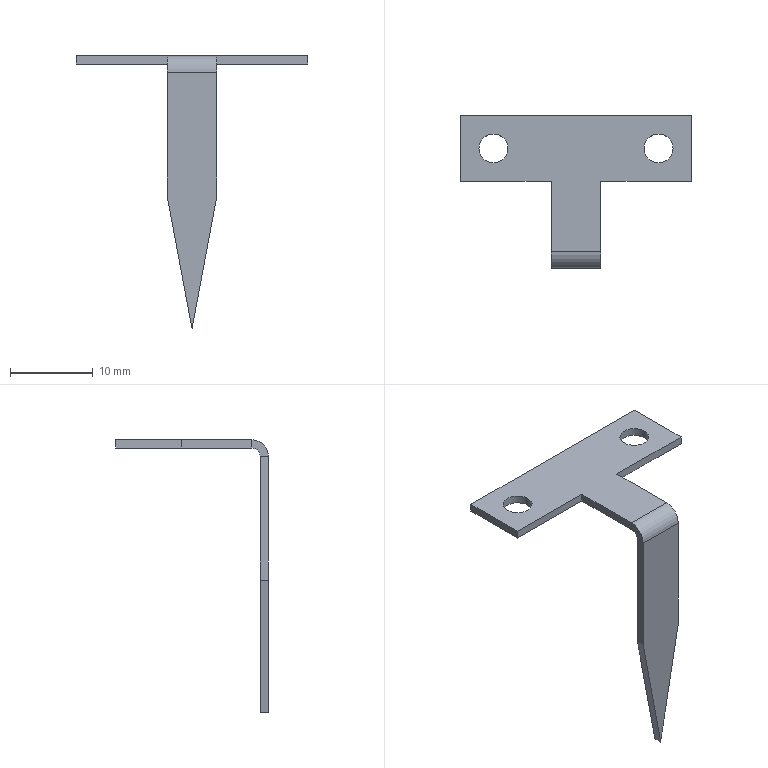Part | SolidWorks | features EdgeFlange 1, FlatPattern 1, SMBaseFlange 1, SheetMetal 1 | 1 solid | 23 faces | box 28 x 18.5 x 33 mm | volume 407.895 mm3 | plane 17 | cylinder 6 | commonest cylinder face diameters 3.5 x4 2 x1 4 x1
STEP:
#1=CARTESIAN_POINT('',(22.25,-4.,-1.));
#2=VERTEX_POINT('',#1);
#3=CARTESIAN_POINT('',(25.75,-4.,-1.));
#4=VERTEX_POINT('',#3);
#5=CARTESIAN_POINT('',(24.,-4.,-1.));
#6=DIRECTION('',(0.,0.,1.));
#7=DIRECTION('',(1.,0.,0.));
#8=AXIS2_PLACEMENT_3D('',#5,#6,#7);
#9=CIRCLE('',#8,1.75);
#10=EDGE_CURVE('',#2,#4,#9,.T.);
#11=ORIENTED_EDGE('',*,*,#10,.F.);
#12=CARTESIAN_POINT('',(22.25,-4.,0.));
#13=VERTEX_POINT('',#12);
#14=CARTESIAN_POINT('',(22.25,-4.,-1.));
#15=DIRECTION('',(0.,0.,1.));
#16=VECTOR('',#15,1000.);
#17=LINE('',#14,#16);
#18=EDGE_CURVE('',#2,#13,#17,.T.);
#19=ORIENTED_EDGE('',*,*,#18,.T.);
#20=CARTESIAN_POINT('',(25.75,-4.,0.));
#21=VERTEX_POINT('',#20);
#22=CARTESIAN_POINT('',(24.,-4.,0.));
#23=DIRECTION('',(0.,0.,1.));
#24=DIRECTION('',(1.,0.,0.));
#25=AXIS2_PLACEMENT_3D('',#22,#23,#24);
#26=CIRCLE('',#25,1.75);
#27=EDGE_CURVE('',#13,#21,#26,.T.);
#28=ORIENTED_EDGE('',*,*,#27,.T.);
#29=CARTESIAN_POINT('',(25.75,-4.,-1.));
#30=DIRECTION('',(0.,0.,1.));
#31=VECTOR('',#30,1000.);
#32=LINE('',#29,#31);
#33=EDGE_CURVE('',#4,#21,#32,.T.);
#34=ORIENTED_EDGE('',*,*,#33,.F.);
#35=EDGE_LOOP('',(#11,#19,#28,#34));
#36=FACE_OUTER_BOUND('',#35,.T.);
#37=CARTESIAN_POINT('',(24.,-4.,-1.));
#38=DIRECTION('',(0.,0.,1.));
#39=DIRECTION('',(1.,0.,0.));
#40=AXIS2_PLACEMENT_3D('',#37,#38,#39);
#41=CYLINDRICAL_SURFACE('',#40,1.75);
#42=ADVANCED_FACE('',(#36),#41,.F.);
#43=CARTESIAN_POINT('',(2.25,-4.,-1.));
#44=VERTEX_POINT('',#43);
#45=CARTESIAN_POINT('',(5.75,-4.,-1.));
#46=VERTEX_POINT('',#45);
#47=CARTESIAN_POINT('',(4.,-4.,-1.));
#48=DIRECTION('',(0.,0.,1.));
#49=DIRECTION('',(1.,0.,0.));
#50=AXIS2_PLACEMENT_3D('',#47,#48,#49);
#51=CIRCLE('',#50,1.75);
#52=EDGE_CURVE('',#44,#46,#51,.T.);
#53=ORIENTED_EDGE('',*,*,#52,.F.);
#54=CARTESIAN_POINT('',(2.25,-4.,0.));
#55=VERTEX_POINT('',#54);
#56=CARTESIAN_POINT('',(2.25,-4.,-1.));
#57=DIRECTION('',(0.,0.,1.));
#58=VECTOR('',#57,1000.);
#59=LINE('',#56,#58);
#60=EDGE_CURVE('',#44,#55,#59,.T.);
#61=ORIENTED_EDGE('',*,*,#60,.T.);
#62=CARTESIAN_POINT('',(5.75,-4.,0.));
#63=VERTEX_POINT('',#62);
#64=CARTESIAN_POINT('',(4.,-4.,0.));
#65=DIRECTION('',(0.,0.,1.));
#66=DIRECTION('',(1.,0.,0.));
#67=AXIS2_PLACEMENT_3D('',#64,#65,#66);
#68=CIRCLE('',#67,1.75);
#69=EDGE_CURVE('',#55,#63,#68,.T.);
#70=ORIENTED_EDGE('',*,*,#69,.T.);
#71=CARTESIAN_POINT('',(5.75,-4.,-1.));
#72=DIRECTION('',(0.,0.,1.));
#73=VECTOR('',#72,1000.);
#74=LINE('',#71,#73);
#75=EDGE_CURVE('',#46,#63,#74,.T.);
#76=ORIENTED_EDGE('',*,*,#75,.F.);
#77=EDGE_LOOP('',(#53,#61,#70,#76));
#78=FACE_OUTER_BOUND('',#77,.T.);
#79=CARTESIAN_POINT('',(4.,-4.,-1.));
#80=DIRECTION('',(0.,0.,1.));
#81=DIRECTION('',(1.,0.,0.));
#82=AXIS2_PLACEMENT_3D('',#79,#80,#81);
#83=CYLINDRICAL_SURFACE('',#82,1.75);
#84=ADVANCED_FACE('',(#78),#83,.F.);
#85=CARTESIAN_POINT('',(11.,-8.,-1.));
#86=VERTEX_POINT('',#85);
#87=CARTESIAN_POINT('',(11.,-16.5,-1.));
#88=VERTEX_POINT('',#87);
#89=CARTESIAN_POINT('',(11.,-8.,-1.));
#90=DIRECTION('',(0.,-1.,0.));
#91=VECTOR('',#90,1000.);
#92=LINE('',#89,#91);
#93=EDGE_CURVE('',#86,#88,#92,.T.);
#94=ORIENTED_EDGE('',*,*,#93,.T.);
#95=CARTESIAN_POINT('',(11.,-16.5,0.));
#96=VERTEX_POINT('',#95);
#97=CARTESIAN_POINT('',(11.,-16.5,-1.));
#98=DIRECTION('',(0.,0.,1.));
#99=VECTOR('',#98,1000.);
#100=LINE('',#97,#99);
#101=EDGE_CURVE('',#88,#96,#100,.T.);
#102=ORIENTED_EDGE('',*,*,#101,.T.);
#103=CARTESIAN_POINT('',(11.,-8.,0.));
#104=VERTEX_POINT('',#103);
#105=CARTESIAN_POINT('',(11.,-8.,0.));
#106=DIRECTION('',(0.,-1.,0.));
#107=VECTOR('',#106,1000.);
#108=LINE('',#105,#107);
#109=EDGE_CURVE('',#104,#96,#108,.T.);
#110=ORIENTED_EDGE('',*,*,#109,.F.);
#111=CARTESIAN_POINT('',(11.,-8.,-1.));
#112=DIRECTION('',(0.,0.,1.));
#113=VECTOR('',#112,1000.);
#114=LINE('',#111,#113);
#115=EDGE_CURVE('',#86,#104,#114,.T.);
#116=ORIENTED_EDGE('',*,*,#115,.F.);
#117=EDGE_LOOP('',(#94,#102,#110,#116));
#118=FACE_OUTER_BOUND('',#117,.T.);
#119=CARTESIAN_POINT('',(11.,-8.,-1.));
#120=DIRECTION('',(-1.,0.,0.));
#121=DIRECTION('',(0.,-1.,0.));
#122=AXIS2_PLACEMENT_3D('',#119,#120,#121);
#123=PLANE('',#122);
#124=ADVANCED_FACE('',(#118),#123,.T.);
#125=CARTESIAN_POINT('',(4.,-4.,-1.));
#126=DIRECTION('',(0.,0.,1.));
#127=DIRECTION('',(1.,0.,0.));
#128=AXIS2_PLACEMENT_3D('',#125,#126,#127);
#129=CIRCLE('',#128,1.75);
#130=EDGE_CURVE('',#46,#44,#129,.T.);
#131=ORIENTED_EDGE('',*,*,#130,.T.);
#132=ORIENTED_EDGE('',*,*,#52,.T.);
#133=EDGE_LOOP('',(#131,#132));
#134=FACE_BOUND('',#133,.T.);
#135=CARTESIAN_POINT('',(24.,-4.,-1.));
#136=DIRECTION('',(0.,0.,1.));
#137=DIRECTION('',(1.,0.,0.));
#138=AXIS2_PLACEMENT_3D('',#135,#136,#137);
#139=CIRCLE('',#138,1.75);
#140=EDGE_CURVE('',#4,#2,#139,.T.);
#141=ORIENTED_EDGE('',*,*,#140,.T.);
#142=ORIENTED_EDGE('',*,*,#10,.T.);
#143=EDGE_LOOP('',(#141,#142));
#144=FACE_BOUND('',#143,.T.);
#145=CARTESIAN_POINT('',(17.,-16.5,-1.));
#146=VERTEX_POINT('',#145);
#147=CARTESIAN_POINT('',(11.,-16.5,-1.));
#148=DIRECTION('',(1.,0.,0.));
#149=VECTOR('',#148,1000.);
#150=LINE('',#147,#149);
#151=EDGE_CURVE('',#88,#146,#150,.T.);
#152=ORIENTED_EDGE('',*,*,#151,.F.);
#153=ORIENTED_EDGE('',*,*,#93,.F.);
#154=CARTESIAN_POINT('',(0.,-8.,-1.));
#155=VERTEX_POINT('',#154);
#156=CARTESIAN_POINT('',(0.,-8.,-1.));
#157=DIRECTION('',(1.,0.,0.));
#158=VECTOR('',#157,1000.);
#159=LINE('',#156,#158);
#160=EDGE_CURVE('',#155,#86,#159,.T.);
#161=ORIENTED_EDGE('',*,*,#160,.F.);
#162=CARTESIAN_POINT('',(0.,0.,-1.));
#163=VERTEX_POINT('',#162);
#164=CARTESIAN_POINT('',(0.,0.,-1.));
#165=DIRECTION('',(0.,-1.,0.));
#166=VECTOR('',#165,1000.);
#167=LINE('',#164,#166);
#168=EDGE_CURVE('',#163,#155,#167,.T.);
#169=ORIENTED_EDGE('',*,*,#168,.F.);
#170=CARTESIAN_POINT('',(28.,0.,-1.));
#171=VERTEX_POINT('',#170);
#172=CARTESIAN_POINT('',(0.,0.,-1.));
#173=DIRECTION('',(-1.,0.,0.));
#174=VECTOR('',#173,1000.);
#175=LINE('',#172,#174);
#176=EDGE_CURVE('',#171,#163,#175,.T.);
#177=ORIENTED_EDGE('',*,*,#176,.F.);
#178=CARTESIAN_POINT('',(28.,-8.,-1.));
#179=VERTEX_POINT('',#178);
#180=CARTESIAN_POINT('',(28.,0.,-1.));
#181=DIRECTION('',(0.,1.,0.));
#182=VECTOR('',#181,1000.);
#183=LINE('',#180,#182);
#184=EDGE_CURVE('',#179,#171,#183,.T.);
#185=ORIENTED_EDGE('',*,*,#184,.F.);
#186=CARTESIAN_POINT('',(17.,-8.,-1.));
#187=VERTEX_POINT('',#186);
#188=CARTESIAN_POINT('',(17.,-8.,-1.));
#189=DIRECTION('',(1.,0.,0.));
#190=VECTOR('',#189,1000.);
#191=LINE('',#188,#190);
#192=EDGE_CURVE('',#187,#179,#191,.T.);
#193=ORIENTED_EDGE('',*,*,#192,.F.);
#194=CARTESIAN_POINT('',(17.,-8.,-1.));
#195=DIRECTION('',(0.,1.,0.));
#196=VECTOR('',#195,1000.);
#197=LINE('',#194,#196);
#198=EDGE_CURVE('',#146,#187,#197,.T.);
#199=ORIENTED_EDGE('',*,*,#198,.F.);
#200=EDGE_LOOP('',(#152,#153,#161,#169,#177,#185,#193,#199));
#201=FACE_OUTER_BOUND('',#200,.T.);
#202=CARTESIAN_POINT('',(0.,0.,-1.));
#203=DIRECTION('',(0.,0.,1.));
#204=DIRECTION('',(1.,0.,0.));
#205=AXIS2_PLACEMENT_3D('',#202,#203,#204);
#206=PLANE('',#205);
#207=ADVANCED_FACE('',(#134,#144,#201),#206,.F.);
#208=CARTESIAN_POINT('',(24.,-4.,0.));
#209=DIRECTION('',(0.,0.,1.));
#210=DIRECTION('',(1.,0.,0.));
#211=AXIS2_PLACEMENT_3D('',#208,#209,#210);
#212=CIRCLE('',#211,1.75);
#213=EDGE_CURVE('',#21,#13,#212,.T.);
#214=ORIENTED_EDGE('',*,*,#213,.F.);
#215=ORIENTED_EDGE('',*,*,#27,.F.);
#216=EDGE_LOOP('',(#214,#215));
#217=FACE_BOUND('',#216,.T.);
#218=CARTESIAN_POINT('',(4.,-4.,0.));
#219=DIRECTION('',(0.,0.,1.));
#220=DIRECTION('',(1.,0.,0.));
#221=AXIS2_PLACEMENT_3D('',#218,#219,#220);
#222=CIRCLE('',#221,1.75);
#223=EDGE_CURVE('',#63,#55,#222,.T.);
#224=ORIENTED_EDGE('',*,*,#223,.F.);
#225=ORIENTED_EDGE('',*,*,#69,.F.);
#226=EDGE_LOOP('',(#224,#225));
#227=FACE_BOUND('',#226,.T.);
#228=ORIENTED_EDGE('',*,*,#109,.T.);
#229=CARTESIAN_POINT('',(17.,-16.5,0.));
#230=VERTEX_POINT('',#229);
#231=CARTESIAN_POINT('',(11.,-16.5,0.));
#232=DIRECTION('',(1.,0.,0.));
#233=VECTOR('',#232,1000.);
#234=LINE('',#231,#233);
#235=EDGE_CURVE('',#96,#230,#234,.T.);
#236=ORIENTED_EDGE('',*,*,#235,.T.);
#237=CARTESIAN_POINT('',(17.,-8.,0.));
#238=VERTEX_POINT('',#237);
#239=CARTESIAN_POINT('',(17.,-8.,0.));
#240=DIRECTION('',(0.,1.,0.));
#241=VECTOR('',#240,1000.);
#242=LINE('',#239,#241);
#243=EDGE_CURVE('',#230,#238,#242,.T.);
#244=ORIENTED_EDGE('',*,*,#243,.T.);
#245=CARTESIAN_POINT('',(28.,-8.,0.));
#246=VERTEX_POINT('',#245);
#247=CARTESIAN_POINT('',(17.,-8.,0.));
#248=DIRECTION('',(1.,0.,0.));
#249=VECTOR('',#248,1000.);
#250=LINE('',#247,#249);
#251=EDGE_CURVE('',#238,#246,#250,.T.);
#252=ORIENTED_EDGE('',*,*,#251,.T.);
#253=CARTESIAN_POINT('',(28.,0.,0.));
#254=VERTEX_POINT('',#253);
#255=CARTESIAN_POINT('',(28.,0.,0.));
#256=DIRECTION('',(0.,1.,0.));
#257=VECTOR('',#256,1000.);
#258=LINE('',#255,#257);
#259=EDGE_CURVE('',#246,#254,#258,.T.);
#260=ORIENTED_EDGE('',*,*,#259,.T.);
#261=CARTESIAN_POINT('',(0.,0.,0.));
#262=VERTEX_POINT('',#261);
#263=CARTESIAN_POINT('',(0.,0.,0.));
#264=DIRECTION('',(-1.,0.,0.));
#265=VECTOR('',#264,1000.);
#266=LINE('',#263,#265);
#267=EDGE_CURVE('',#254,#262,#266,.T.);
#268=ORIENTED_EDGE('',*,*,#267,.T.);
#269=CARTESIAN_POINT('',(0.,-8.,0.));
#270=VERTEX_POINT('',#269);
#271=CARTESIAN_POINT('',(0.,0.,0.));
#272=DIRECTION('',(0.,-1.,0.));
#273=VECTOR('',#272,1000.);
#274=LINE('',#271,#273);
#275=EDGE_CURVE('',#262,#270,#274,.T.);
#276=ORIENTED_EDGE('',*,*,#275,.T.);
#277=CARTESIAN_POINT('',(0.,-8.,0.));
#278=DIRECTION('',(1.,0.,0.));
#279=VECTOR('',#278,1000.);
#280=LINE('',#277,#279);
#281=EDGE_CURVE('',#270,#104,#280,.T.);
#282=ORIENTED_EDGE('',*,*,#281,.T.);
#283=EDGE_LOOP('',(#228,#236,#244,#252,#260,#268,#276,#282));
#284=FACE_OUTER_BOUND('',#283,.T.);
#285=CARTESIAN_POINT('',(0.,0.,0.));
#286=DIRECTION('',(0.,0.,1.));
#287=DIRECTION('',(1.,0.,0.));
#288=AXIS2_PLACEMENT_3D('',#285,#286,#287);
#289=PLANE('',#288);
#290=ADVANCED_FACE('',(#217,#227,#284),#289,.T.);
#291=ORIENTED_EDGE('',*,*,#275,.F.);
#292=CARTESIAN_POINT('',(0.,0.,-1.));
#293=DIRECTION('',(0.,0.,1.));
#294=VECTOR('',#293,1000.);
#295=LINE('',#292,#294);
#296=EDGE_CURVE('',#163,#262,#295,.T.);
#297=ORIENTED_EDGE('',*,*,#296,.F.);
#298=ORIENTED_EDGE('',*,*,#168,.T.);
#299=CARTESIAN_POINT('',(0.,-8.,-1.));
#300=DIRECTION('',(0.,0.,1.));
#301=VECTOR('',#300,1000.);
#302=LINE('',#299,#301);
#303=EDGE_CURVE('',#155,#270,#302,.T.);
#304=ORIENTED_EDGE('',*,*,#303,.T.);
#305=EDGE_LOOP('',(#291,#297,#298,#304));
#306=FACE_OUTER_BOUND('',#305,.T.);
#307=CARTESIAN_POINT('',(0.,0.,-1.));
#308=DIRECTION('',(-1.,0.,0.));
#309=DIRECTION('',(0.,-1.,0.));
#310=AXIS2_PLACEMENT_3D('',#307,#308,#309);
#311=PLANE('',#310);
#312=ADVANCED_FACE('',(#306),#311,.T.);
#313=ORIENTED_EDGE('',*,*,#267,.F.);
#314=CARTESIAN_POINT('',(28.,0.,-1.));
#315=DIRECTION('',(0.,0.,1.));
#316=VECTOR('',#315,1000.);
#317=LINE('',#314,#316);
#318=EDGE_CURVE('',#171,#254,#317,.T.);
#319=ORIENTED_EDGE('',*,*,#318,.F.);
#320=ORIENTED_EDGE('',*,*,#176,.T.);
#321=ORIENTED_EDGE('',*,*,#296,.T.);
#322=EDGE_LOOP('',(#313,#319,#320,#321));
#323=FACE_OUTER_BOUND('',#322,.T.);
#324=CARTESIAN_POINT('',(0.,0.,-1.));
#325=DIRECTION('',(0.,1.,0.));
#326=DIRECTION('',(-1.,0.,0.));
#327=AXIS2_PLACEMENT_3D('',#324,#325,#326);
#328=PLANE('',#327);
#329=ADVANCED_FACE('',(#323),#328,.T.);
#330=ORIENTED_EDGE('',*,*,#259,.F.);
#331=CARTESIAN_POINT('',(28.,-8.,-1.));
#332=DIRECTION('',(0.,0.,1.));
#333=VECTOR('',#332,1000.);
#334=LINE('',#331,#333);
#335=EDGE_CURVE('',#179,#246,#334,.T.);
#336=ORIENTED_EDGE('',*,*,#335,.F.);
#337=ORIENTED_EDGE('',*,*,#184,.T.);
#338=ORIENTED_EDGE('',*,*,#318,.T.);
#339=EDGE_LOOP('',(#330,#336,#337,#338));
#340=FACE_OUTER_BOUND('',#339,.T.);
#341=CARTESIAN_POINT('',(28.,0.,-1.));
#342=DIRECTION('',(1.,0.,0.));
#343=DIRECTION('',(0.,0.,-1.));
#344=AXIS2_PLACEMENT_3D('',#341,#342,#343);
#345=PLANE('',#344);
#346=ADVANCED_FACE('',(#340),#345,.T.);
#347=ORIENTED_EDGE('',*,*,#251,.F.);
#348=CARTESIAN_POINT('',(17.,-8.,-1.));
#349=DIRECTION('',(0.,0.,1.));
#350=VECTOR('',#349,1000.);
#351=LINE('',#348,#350);
#352=EDGE_CURVE('',#187,#238,#351,.T.);
#353=ORIENTED_EDGE('',*,*,#352,.F.);
#354=ORIENTED_EDGE('',*,*,#192,.T.);
#355=ORIENTED_EDGE('',*,*,#335,.T.);
#356=EDGE_LOOP('',(#347,#353,#354,#355));
#357=FACE_OUTER_BOUND('',#356,.T.);
#358=CARTESIAN_POINT('',(17.,-8.,-1.));
#359=DIRECTION('',(0.,-1.,0.));
#360=DIRECTION('',(1.,0.,0.));
#361=AXIS2_PLACEMENT_3D('',#358,#359,#360);
#362=PLANE('',#361);
#363=ADVANCED_FACE('',(#357),#362,.T.);
#364=CARTESIAN_POINT('',(17.,-16.5,-1.));
#365=DIRECTION('',(0.,0.,1.));
#366=VECTOR('',#365,1000.);
#367=LINE('',#364,#366);
#368=EDGE_CURVE('',#146,#230,#367,.T.);
#369=ORIENTED_EDGE('',*,*,#368,.F.);
#370=ORIENTED_EDGE('',*,*,#198,.T.);
#371=ORIENTED_EDGE('',*,*,#352,.T.);
#372=ORIENTED_EDGE('',*,*,#243,.F.);
#373=EDGE_LOOP('',(#369,#370,#371,#372));
#374=FACE_OUTER_BOUND('',#373,.T.);
#375=CARTESIAN_POINT('',(17.,-8.,-1.));
#376=DIRECTION('',(1.,0.,0.));
#377=DIRECTION('',(0.,0.,-1.));
#378=AXIS2_PLACEMENT_3D('',#375,#376,#377);
#379=PLANE('',#378);
#380=ADVANCED_FACE('',(#374),#379,.T.);
#381=ORIENTED_EDGE('',*,*,#281,.F.);
#382=ORIENTED_EDGE('',*,*,#303,.F.);
#383=ORIENTED_EDGE('',*,*,#160,.T.);
#384=ORIENTED_EDGE('',*,*,#115,.T.);
#385=EDGE_LOOP('',(#381,#382,#383,#384));
#386=FACE_OUTER_BOUND('',#385,.T.);
#387=CARTESIAN_POINT('',(0.,-8.,-1.));
#388=DIRECTION('',(0.,-1.,0.));
#389=DIRECTION('',(1.,0.,0.));
#390=AXIS2_PLACEMENT_3D('',#387,#388,#389);
#391=PLANE('',#390);
#392=ADVANCED_FACE('',(#386),#391,.T.);
#393=ORIENTED_EDGE('',*,*,#60,.F.);
#394=ORIENTED_EDGE('',*,*,#130,.F.);
#395=ORIENTED_EDGE('',*,*,#75,.T.);
#396=ORIENTED_EDGE('',*,*,#223,.T.);
#397=EDGE_LOOP('',(#393,#394,#395,#396));
#398=FACE_OUTER_BOUND('',#397,.T.);
#399=CARTESIAN_POINT('',(4.,-4.,-1.));
#400=DIRECTION('',(0.,0.,1.));
#401=DIRECTION('',(1.,0.,0.));
#402=AXIS2_PLACEMENT_3D('',#399,#400,#401);
#403=CYLINDRICAL_SURFACE('',#402,1.75);
#404=ADVANCED_FACE('',(#398),#403,.F.);
#405=ORIENTED_EDGE('',*,*,#18,.F.);
#406=ORIENTED_EDGE('',*,*,#140,.F.);
#407=ORIENTED_EDGE('',*,*,#33,.T.);
#408=ORIENTED_EDGE('',*,*,#213,.T.);
#409=EDGE_LOOP('',(#405,#406,#407,#408));
#410=FACE_OUTER_BOUND('',#409,.T.);
#411=CARTESIAN_POINT('',(24.,-4.,-1.));
#412=DIRECTION('',(0.,0.,1.));
#413=DIRECTION('',(1.,0.,0.));
#414=AXIS2_PLACEMENT_3D('',#411,#412,#413);
#415=CYLINDRICAL_SURFACE('',#414,1.75);
#416=ADVANCED_FACE('',(#410),#415,.F.);
#417=CARTESIAN_POINT('',(17.,-17.5,-2.));
#418=VERTEX_POINT('',#417);
#419=CARTESIAN_POINT('',(17.,-18.5,-2.));
#420=VERTEX_POINT('',#419);
#421=CARTESIAN_POINT('',(17.,-18.5,-2.));
#422=DIRECTION('',(0.,-1.,0.));
#423=VECTOR('',#422,1000.);
#424=LINE('',#421,#423);
#425=EDGE_CURVE('',#418,#420,#424,.T.);
#426=ORIENTED_EDGE('',*,*,#425,.F.);
#427=CARTESIAN_POINT('',(17.,-16.5,-2.));
#428=DIRECTION('',(1.,0.,0.));
#429=DIRECTION('',(0.,0.,1.));
#430=AXIS2_PLACEMENT_3D('',#427,#428,#429);
#431=CIRCLE('',#430,1.);
#432=EDGE_CURVE('',#146,#418,#431,.T.);
#433=ORIENTED_EDGE('',*,*,#432,.F.);
#434=ORIENTED_EDGE('',*,*,#368,.T.);
#435=CARTESIAN_POINT('',(17.,-16.5,-2.));
#436=DIRECTION('',(1.,0.,0.));
#437=DIRECTION('',(0.,0.,1.));
#438=AXIS2_PLACEMENT_3D('',#435,#436,#437);
#439=CIRCLE('',#438,2.);
#440=EDGE_CURVE('',#230,#420,#439,.T.);
#441=ORIENTED_EDGE('',*,*,#440,.T.);
#442=EDGE_LOOP('',(#426,#433,#434,#441));
#443=FACE_OUTER_BOUND('',#442,.T.);
#444=CARTESIAN_POINT('',(17.,-16.5,-2.));
#445=DIRECTION('',(1.,0.,0.));
#446=DIRECTION('',(0.,0.,-1.));
#447=AXIS2_PLACEMENT_3D('',#444,#445,#446);
#448=PLANE('',#447);
#449=ADVANCED_FACE('',(#443),#448,.T.);
#450=CARTESIAN_POINT('',(11.,-17.5,-2.));
#451=VERTEX_POINT('',#450);
#452=CARTESIAN_POINT('',(11.,-16.5,-2.));
#453=DIRECTION('',(-1.,0.,0.));
#454=DIRECTION('',(0.,0.,1.));
#455=AXIS2_PLACEMENT_3D('',#452,#453,#454);
#456=CIRCLE('',#455,1.);
#457=EDGE_CURVE('',#451,#88,#456,.T.);
#458=ORIENTED_EDGE('',*,*,#457,.F.);
#459=CARTESIAN_POINT('',(11.,-18.5,-2.));
#460=VERTEX_POINT('',#459);
#461=CARTESIAN_POINT('',(11.,-17.5,-2.));
#462=DIRECTION('',(0.,-1.,0.));
#463=VECTOR('',#462,1000.);
#464=LINE('',#461,#463);
#465=EDGE_CURVE('',#451,#460,#464,.T.);
#466=ORIENTED_EDGE('',*,*,#465,.T.);
#467=CARTESIAN_POINT('',(11.,-16.5,-2.));
#468=DIRECTION('',(-1.,0.,0.));
#469=DIRECTION('',(0.,0.,1.));
#470=AXIS2_PLACEMENT_3D('',#467,#468,#469);
#471=CIRCLE('',#470,2.);
#472=EDGE_CURVE('',#460,#96,#471,.T.);
#473=ORIENTED_EDGE('',*,*,#472,.T.);
#474=ORIENTED_EDGE('',*,*,#101,.F.);
#475=EDGE_LOOP('',(#458,#466,#473,#474));
#476=FACE_OUTER_BOUND('',#475,.T.);
#477=CARTESIAN_POINT('',(11.,-16.5,-2.));
#478=DIRECTION('',(1.,0.,0.));
#479=DIRECTION('',(0.,0.,-1.));
#480=AXIS2_PLACEMENT_3D('',#477,#478,#479);
#481=PLANE('',#480);
#482=ADVANCED_FACE('',(#476),#481,.F.);
#483=ORIENTED_EDGE('',*,*,#235,.F.);
#484=ORIENTED_EDGE('',*,*,#472,.F.);
#485=CARTESIAN_POINT('',(17.,-18.5,-2.));
#486=DIRECTION('',(1.,0.,0.));
#487=VECTOR('',#486,1000.);
#488=LINE('',#485,#487);
#489=EDGE_CURVE('',#460,#420,#488,.T.);
#490=ORIENTED_EDGE('',*,*,#489,.T.);
#491=ORIENTED_EDGE('',*,*,#440,.F.);
#492=EDGE_LOOP('',(#483,#484,#490,#491));
#493=FACE_OUTER_BOUND('',#492,.T.);
#494=CARTESIAN_POINT('',(11.,-16.5,-2.));
#495=DIRECTION('',(-1.,0.,0.));
#496=DIRECTION('',(0.,-1.,0.));
#497=AXIS2_PLACEMENT_3D('',#494,#495,#496);
#498=CYLINDRICAL_SURFACE('',#497,2.);
#499=ADVANCED_FACE('',(#493),#498,.T.);
#500=ORIENTED_EDGE('',*,*,#151,.T.);
#501=ORIENTED_EDGE('',*,*,#432,.T.);
#502=CARTESIAN_POINT('',(17.,-17.5,-2.));
#503=DIRECTION('',(-1.,0.,0.));
#504=VECTOR('',#503,1000.);
#505=LINE('',#502,#504);
#506=EDGE_CURVE('',#418,#451,#505,.T.);
#507=ORIENTED_EDGE('',*,*,#506,.T.);
#508=ORIENTED_EDGE('',*,*,#457,.T.);
#509=EDGE_LOOP('',(#500,#501,#507,#508));
#510=FACE_OUTER_BOUND('',#509,.T.);
#511=CARTESIAN_POINT('',(11.,-16.5,-2.));
#512=DIRECTION('',(-1.,0.,0.));
#513=DIRECTION('',(0.,-1.,0.));
#514=AXIS2_PLACEMENT_3D('',#511,#512,#513);
#515=CYLINDRICAL_SURFACE('',#514,1.);
#516=ADVANCED_FACE('',(#510),#515,.F.);
#517=ORIENTED_EDGE('',*,*,#465,.F.);
#518=CARTESIAN_POINT('',(11.,-17.5,-17.));
#519=VERTEX_POINT('',#518);
#520=CARTESIAN_POINT('',(11.,-17.5,-17.));
#521=DIRECTION('',(0.,0.,-1.));
#522=VECTOR('',#521,1000.);
#523=LINE('',#520,#522);
#524=EDGE_CURVE('',#451,#519,#523,.T.);
#525=ORIENTED_EDGE('',*,*,#524,.T.);
#526=CARTESIAN_POINT('',(11.,-18.5,-17.));
#527=VERTEX_POINT('',#526);
#528=CARTESIAN_POINT('',(11.,-18.5,-17.));
#529=DIRECTION('',(0.,1.,0.));
#530=VECTOR('',#529,1000.);
#531=LINE('',#528,#530);
#532=EDGE_CURVE('',#527,#519,#531,.T.);
#533=ORIENTED_EDGE('',*,*,#532,.F.);
#534=CARTESIAN_POINT('',(11.,-18.5,0.));
#535=DIRECTION('',(0.,0.,-1.));
#536=VECTOR('',#535,1000.);
#537=LINE('',#534,#536);
#538=EDGE_CURVE('',#460,#527,#537,.T.);
#539=ORIENTED_EDGE('',*,*,#538,.F.);
#540=EDGE_LOOP('',(#517,#525,#533,#539));
#541=FACE_OUTER_BOUND('',#540,.T.);
#542=CARTESIAN_POINT('',(11.,-18.5,-17.));
#543=DIRECTION('',(1.,0.,0.));
#544=DIRECTION('',(0.,0.,-1.));
#545=AXIS2_PLACEMENT_3D('',#542,#543,#544);
#546=PLANE('',#545);
#547=ADVANCED_FACE('',(#541),#546,.F.);
#548=ORIENTED_EDGE('',*,*,#425,.T.);
#549=CARTESIAN_POINT('',(17.,-18.5,-17.));
#550=VERTEX_POINT('',#549);
#551=CARTESIAN_POINT('',(17.,-18.5,0.));
#552=DIRECTION('',(0.,0.,1.));
#553=VECTOR('',#552,1000.);
#554=LINE('',#551,#553);
#555=EDGE_CURVE('',#550,#420,#554,.T.);
#556=ORIENTED_EDGE('',*,*,#555,.F.);
#557=CARTESIAN_POINT('',(17.,-17.5,-17.));
#558=VERTEX_POINT('',#557);
#559=CARTESIAN_POINT('',(17.,-18.5,-17.));
#560=DIRECTION('',(0.,1.,0.));
#561=VECTOR('',#560,1000.);
#562=LINE('',#559,#561);
#563=EDGE_CURVE('',#550,#558,#562,.T.);
#564=ORIENTED_EDGE('',*,*,#563,.T.);
#565=CARTESIAN_POINT('',(17.,-17.5,-1.));
#566=DIRECTION('',(0.,0.,1.));
#567=VECTOR('',#566,1000.);
#568=LINE('',#565,#567);
#569=EDGE_CURVE('',#558,#418,#568,.T.);
#570=ORIENTED_EDGE('',*,*,#569,.T.);
#571=EDGE_LOOP('',(#548,#556,#564,#570));
#572=FACE_OUTER_BOUND('',#571,.T.);
#573=CARTESIAN_POINT('',(17.,-18.5,-1.));
#574=DIRECTION('',(-1.,0.,0.));
#575=DIRECTION('',(0.,0.,1.));
#576=AXIS2_PLACEMENT_3D('',#573,#574,#575);
#577=PLANE('',#576);
#578=ADVANCED_FACE('',(#572),#577,.F.);
#579=ORIENTED_EDGE('',*,*,#489,.F.);
#580=ORIENTED_EDGE('',*,*,#538,.T.);
#581=CARTESIAN_POINT('',(14.,-18.5,-33.));
#582=VERTEX_POINT('',#581);
#583=CARTESIAN_POINT('',(7.547,-18.5,1.415));
#584=DIRECTION('',(0.1843,0.,-0.9829));
#585=VECTOR('',#584,1000.);
#586=LINE('',#583,#585);
#587=EDGE_CURVE('',#527,#582,#586,.T.);
#588=ORIENTED_EDGE('',*,*,#587,.T.);
#589=CARTESIAN_POINT('',(19.502,-18.5,-3.657));
#590=DIRECTION('',(0.1843,0.,0.9829));
#591=VECTOR('',#590,1000.);
#592=LINE('',#589,#591);
#593=EDGE_CURVE('',#582,#550,#592,.T.);
#594=ORIENTED_EDGE('',*,*,#593,.T.);
#595=ORIENTED_EDGE('',*,*,#555,.T.);
#596=EDGE_LOOP('',(#579,#580,#588,#594,#595));
#597=FACE_OUTER_BOUND('',#596,.T.);
#598=CARTESIAN_POINT('',(0.,-18.5,0.));
#599=DIRECTION('',(0.,1.,0.));
#600=DIRECTION('',(0.,0.,1.));
#601=AXIS2_PLACEMENT_3D('',#598,#599,#600);
#602=PLANE('',#601);
#603=ADVANCED_FACE('',(#597),#602,.F.);
#604=ORIENTED_EDGE('',*,*,#524,.F.);
#605=ORIENTED_EDGE('',*,*,#506,.F.);
#606=ORIENTED_EDGE('',*,*,#569,.F.);
#607=CARTESIAN_POINT('',(14.,-17.5,-33.));
#608=VERTEX_POINT('',#607);
#609=CARTESIAN_POINT('',(14.,-17.5,-33.));
#610=DIRECTION('',(0.1843,0.,0.9829));
#611=VECTOR('',#610,1000.);
#612=LINE('',#609,#611);
#613=EDGE_CURVE('',#608,#558,#612,.T.);
#614=ORIENTED_EDGE('',*,*,#613,.F.);
#615=CARTESIAN_POINT('',(11.,-17.5,-17.));
#616=DIRECTION('',(0.1843,0.,-0.9829));
#617=VECTOR('',#616,1000.);
#618=LINE('',#615,#617);
#619=EDGE_CURVE('',#519,#608,#618,.T.);
#620=ORIENTED_EDGE('',*,*,#619,.F.);
#621=EDGE_LOOP('',(#604,#605,#606,#614,#620));
#622=FACE_OUTER_BOUND('',#621,.T.);
#623=CARTESIAN_POINT('',(0.,-17.5,0.));
#624=DIRECTION('',(0.,1.,0.));
#625=DIRECTION('',(0.,0.,1.));
#626=AXIS2_PLACEMENT_3D('',#623,#624,#625);
#627=PLANE('',#626);
#628=ADVANCED_FACE('',(#622),#627,.T.);
#629=ORIENTED_EDGE('',*,*,#619,.T.);
#630=CARTESIAN_POINT('',(14.,-18.5,-33.));
#631=DIRECTION('',(0.,1.,0.));
#632=VECTOR('',#631,1000.);
#633=LINE('',#630,#632);
#634=EDGE_CURVE('',#582,#608,#633,.T.);
#635=ORIENTED_EDGE('',*,*,#634,.F.);
#636=ORIENTED_EDGE('',*,*,#587,.F.);
#637=ORIENTED_EDGE('',*,*,#532,.T.);
#638=EDGE_LOOP('',(#629,#635,#636,#637));
#639=FACE_OUTER_BOUND('',#638,.T.);
#640=CARTESIAN_POINT('',(11.,-18.5,-17.));
#641=DIRECTION('',(0.9829,0.,0.1843));
#642=DIRECTION('',(0.1843,0.,-0.9829));
#643=AXIS2_PLACEMENT_3D('',#640,#641,#642);
#644=PLANE('',#643);
#645=ADVANCED_FACE('',(#639),#644,.F.);
#646=ORIENTED_EDGE('',*,*,#613,.T.);
#647=ORIENTED_EDGE('',*,*,#563,.F.);
#648=ORIENTED_EDGE('',*,*,#593,.F.);
#649=ORIENTED_EDGE('',*,*,#634,.T.);
#650=EDGE_LOOP('',(#646,#647,#648,#649));
#651=FACE_OUTER_BOUND('',#650,.T.);
#652=CARTESIAN_POINT('',(14.,-18.5,-33.));
#653=DIRECTION('',(-0.9829,0.,0.1843));
#654=DIRECTION('',(0.1843,0.,0.9829));
#655=AXIS2_PLACEMENT_3D('',#652,#653,#654);
#656=PLANE('',#655);
#657=ADVANCED_FACE('',(#651),#656,.F.);
#658=CLOSED_SHELL('',(#42,#84,#124,#207,#290,#312,#329,#346,#363,#380,#392,#404,#416,#449,#482,#499,#516,#547,#578,#603,#628,#645,#657));
#659=MANIFOLD_SOLID_BREP('',#658);
#660=CARTESIAN_POINT('',(0.,0.,0.));
#661=DIRECTION('',(0.,0.,1.));
#662=DIRECTION('',(1.,0.,0.));
#663=AXIS2_PLACEMENT_3D('',#660,#661,#662);
#664=(LENGTH_UNIT()NAMED_UNIT(*)SI_UNIT(.MILLI.,.METRE.));
#665=UNCERTAINTY_MEASURE_WITH_UNIT(LENGTH_MEASURE(0.00001),#664,'','');
#666=(NAMED_UNIT(*)PLANE_ANGLE_UNIT()SI_UNIT($,.RADIAN.));
#667=(NAMED_UNIT(*)SI_UNIT($,.STERADIAN.)SOLID_ANGLE_UNIT());
#668=(GEOMETRIC_REPRESENTATION_CONTEXT(3)GLOBAL_UNCERTAINTY_ASSIGNED_CONTEXT((#665))GLOBAL_UNIT_ASSIGNED_CONTEXT((#664,#666,#667))REPRESENTATION_CONTEXT('',''));
#669=ADVANCED_BREP_SHAPE_REPRESENTATION('',(#659,#663),#668);